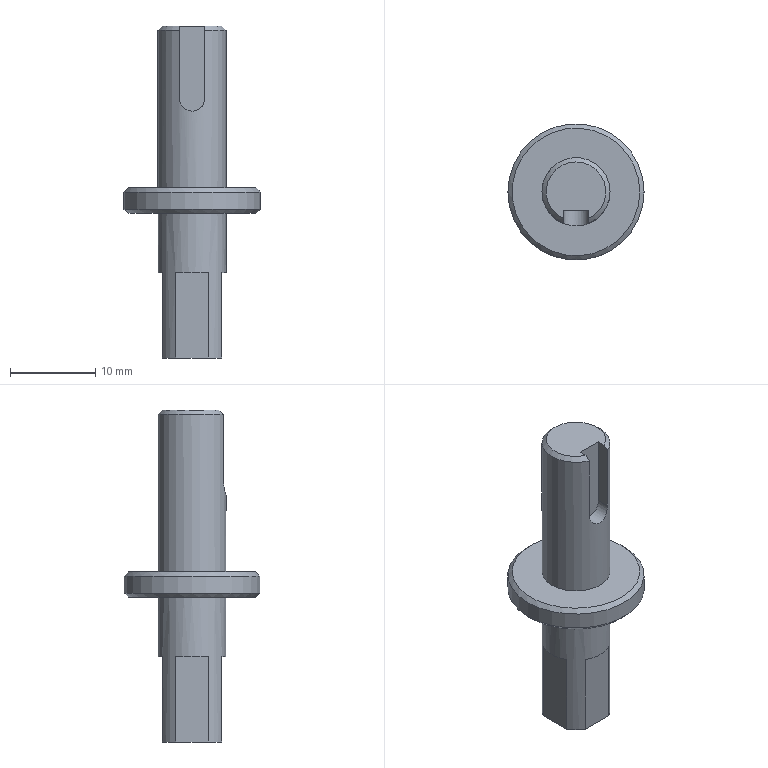Part | NX | features DATUM_CSYS 2, EXTRUDE 2, BREP 1, SKETCH 1 | 1 solid | 25 faces | box 16 x 16 x 39 mm | volume 2221 mm3 | plane 15 | cylinder 6 | cone 4 | commonest cylinder face diameters 2.5 x2 8 x2 3 x1 16 x1
STEP:
#1=CARTESIAN_POINT('',(-3.5,1.936,-20.));
#2=VERTEX_POINT('',#1);
#3=CARTESIAN_POINT('',(-1.936,3.5,-20.));
#4=VERTEX_POINT('',#3);
#5=CARTESIAN_POINT('',(0.,0.,-20.));
#6=DIRECTION('',(0.,0.,-1.));
#7=DIRECTION('',(1.,0.,0.));
#8=AXIS2_PLACEMENT_3D('',#5,#6,#7);
#9=CIRCLE('',#8,4.);
#10=EDGE_CURVE('',#2,#4,#9,.T.);
#11=ORIENTED_EDGE('',*,*,#10,.F.);
#12=CARTESIAN_POINT('',(-3.5,1.936,-10.));
#13=VERTEX_POINT('',#12);
#14=CARTESIAN_POINT('',(-3.5,1.936,-10.));
#15=DIRECTION('',(0.,0.,-1.));
#16=VECTOR('',#15,1000.);
#17=LINE('',#14,#16);
#18=EDGE_CURVE('',#13,#2,#17,.T.);
#19=ORIENTED_EDGE('',*,*,#18,.F.);
#20=CARTESIAN_POINT('',(-3.5,-1.936,-10.));
#21=VERTEX_POINT('',#20);
#22=CARTESIAN_POINT('',(0.,0.,-10.));
#23=DIRECTION('',(0.,0.,-1.));
#24=DIRECTION('',(-0.875,-0.4841,0.));
#25=AXIS2_PLACEMENT_3D('',#22,#23,#24);
#26=CIRCLE('',#25,4.);
#27=EDGE_CURVE('',#21,#13,#26,.T.);
#28=ORIENTED_EDGE('',*,*,#27,.F.);
#29=CARTESIAN_POINT('',(-3.5,-1.936,-20.));
#30=VERTEX_POINT('',#29);
#31=CARTESIAN_POINT('',(-3.5,-1.936,-14.5));
#32=DIRECTION('',(0.,0.,1.));
#33=VECTOR('',#32,1000.);
#34=LINE('',#31,#33);
#35=EDGE_CURVE('',#30,#21,#34,.T.);
#36=ORIENTED_EDGE('',*,*,#35,.F.);
#37=CARTESIAN_POINT('',(-1.936,-3.5,-20.));
#38=VERTEX_POINT('',#37);
#39=CARTESIAN_POINT('',(0.,0.,-20.));
#40=DIRECTION('',(0.,0.,-1.));
#41=DIRECTION('',(1.,0.,0.));
#42=AXIS2_PLACEMENT_3D('',#39,#40,#41);
#43=CIRCLE('',#42,4.);
#44=EDGE_CURVE('',#38,#30,#43,.T.);
#45=ORIENTED_EDGE('',*,*,#44,.F.);
#46=CARTESIAN_POINT('',(-1.936,-3.5,-10.));
#47=VERTEX_POINT('',#46);
#48=CARTESIAN_POINT('',(-1.936,-3.5,-10.));
#49=DIRECTION('',(0.,0.,-1.));
#50=VECTOR('',#49,1000.);
#51=LINE('',#48,#50);
#52=EDGE_CURVE('',#47,#38,#51,.T.);
#53=ORIENTED_EDGE('',*,*,#52,.F.);
#54=CARTESIAN_POINT('',(1.936,-3.5,-10.));
#55=VERTEX_POINT('',#54);
#56=CARTESIAN_POINT('',(0.,0.,-10.));
#57=DIRECTION('',(0.,0.,-1.));
#58=DIRECTION('',(0.4841,-0.875,0.));
#59=AXIS2_PLACEMENT_3D('',#56,#57,#58);
#60=CIRCLE('',#59,4.);
#61=EDGE_CURVE('',#55,#47,#60,.T.);
#62=ORIENTED_EDGE('',*,*,#61,.F.);
#63=CARTESIAN_POINT('',(1.936,-3.5,-20.));
#64=VERTEX_POINT('',#63);
#65=CARTESIAN_POINT('',(1.936,-3.5,-14.5));
#66=DIRECTION('',(0.,0.,1.));
#67=VECTOR('',#66,1000.);
#68=LINE('',#65,#67);
#69=EDGE_CURVE('',#64,#55,#68,.T.);
#70=ORIENTED_EDGE('',*,*,#69,.F.);
#71=CARTESIAN_POINT('',(3.5,-1.936,-20.));
#72=VERTEX_POINT('',#71);
#73=CARTESIAN_POINT('',(0.,0.,-20.));
#74=DIRECTION('',(0.,0.,-1.));
#75=DIRECTION('',(1.,0.,0.));
#76=AXIS2_PLACEMENT_3D('',#73,#74,#75);
#77=CIRCLE('',#76,4.);
#78=EDGE_CURVE('',#72,#64,#77,.T.);
#79=ORIENTED_EDGE('',*,*,#78,.F.);
#80=CARTESIAN_POINT('',(3.5,-1.936,-10.));
#81=VERTEX_POINT('',#80);
#82=CARTESIAN_POINT('',(3.5,-1.936,-10.));
#83=DIRECTION('',(0.,0.,-1.));
#84=VECTOR('',#83,1000.);
#85=LINE('',#82,#84);
#86=EDGE_CURVE('',#81,#72,#85,.T.);
#87=ORIENTED_EDGE('',*,*,#86,.F.);
#88=CARTESIAN_POINT('',(4.,0.,-10.));
#89=VERTEX_POINT('',#88);
#90=CARTESIAN_POINT('',(0.,0.,-10.));
#91=DIRECTION('',(0.,0.,-1.));
#92=DIRECTION('',(1.,0.,0.));
#93=AXIS2_PLACEMENT_3D('',#90,#91,#92);
#94=CIRCLE('',#93,4.);
#95=EDGE_CURVE('',#89,#81,#94,.T.);
#96=ORIENTED_EDGE('',*,*,#95,.F.);
#97=CARTESIAN_POINT('',(4.,0.,-3.));
#98=VERTEX_POINT('',#97);
#99=CARTESIAN_POINT('',(4.,0.,-3.));
#100=DIRECTION('',(0.,0.,-1.));
#101=VECTOR('',#100,1000.);
#102=LINE('',#99,#101);
#103=EDGE_CURVE('',#98,#89,#102,.T.);
#104=ORIENTED_EDGE('',*,*,#103,.F.);
#105=CARTESIAN_POINT('',(0.,0.,-3.));
#106=DIRECTION('',(0.,0.,-1.));
#107=DIRECTION('',(1.,0.,0.));
#108=AXIS2_PLACEMENT_3D('',#105,#106,#107);
#109=CIRCLE('',#108,4.);
#110=EDGE_CURVE('',#98,#98,#109,.T.);
#111=ORIENTED_EDGE('',*,*,#110,.T.);
#112=ORIENTED_EDGE('',*,*,#103,.T.);
#113=CARTESIAN_POINT('',(3.5,1.936,-10.));
#114=VERTEX_POINT('',#113);
#115=CARTESIAN_POINT('',(0.,0.,-10.));
#116=DIRECTION('',(0.,0.,-1.));
#117=DIRECTION('',(0.875,0.4841,0.));
#118=AXIS2_PLACEMENT_3D('',#115,#116,#117);
#119=CIRCLE('',#118,4.);
#120=EDGE_CURVE('',#114,#89,#119,.T.);
#121=ORIENTED_EDGE('',*,*,#120,.F.);
#122=CARTESIAN_POINT('',(3.5,1.936,-20.));
#123=VERTEX_POINT('',#122);
#124=CARTESIAN_POINT('',(3.5,1.936,-14.5));
#125=DIRECTION('',(0.,0.,1.));
#126=VECTOR('',#125,1000.);
#127=LINE('',#124,#126);
#128=EDGE_CURVE('',#123,#114,#127,.T.);
#129=ORIENTED_EDGE('',*,*,#128,.F.);
#130=CARTESIAN_POINT('',(1.936,3.5,-20.));
#131=VERTEX_POINT('',#130);
#132=CARTESIAN_POINT('',(0.,0.,-20.));
#133=DIRECTION('',(0.,0.,-1.));
#134=DIRECTION('',(1.,0.,0.));
#135=AXIS2_PLACEMENT_3D('',#132,#133,#134);
#136=CIRCLE('',#135,4.);
#137=EDGE_CURVE('',#131,#123,#136,.T.);
#138=ORIENTED_EDGE('',*,*,#137,.F.);
#139=CARTESIAN_POINT('',(1.936,3.5,-10.));
#140=VERTEX_POINT('',#139);
#141=CARTESIAN_POINT('',(1.936,3.5,-10.));
#142=DIRECTION('',(0.,0.,-1.));
#143=VECTOR('',#142,1000.);
#144=LINE('',#141,#143);
#145=EDGE_CURVE('',#140,#131,#144,.T.);
#146=ORIENTED_EDGE('',*,*,#145,.F.);
#147=CARTESIAN_POINT('',(-1.936,3.5,-10.));
#148=VERTEX_POINT('',#147);
#149=CARTESIAN_POINT('',(0.,0.,-10.));
#150=DIRECTION('',(0.,0.,-1.));
#151=DIRECTION('',(-0.4841,0.875,0.));
#152=AXIS2_PLACEMENT_3D('',#149,#150,#151);
#153=CIRCLE('',#152,4.);
#154=EDGE_CURVE('',#148,#140,#153,.T.);
#155=ORIENTED_EDGE('',*,*,#154,.F.);
#156=CARTESIAN_POINT('',(-1.936,3.5,-14.5));
#157=DIRECTION('',(0.,0.,1.));
#158=VECTOR('',#157,1000.);
#159=LINE('',#156,#158);
#160=EDGE_CURVE('',#4,#148,#159,.T.);
#161=ORIENTED_EDGE('',*,*,#160,.F.);
#162=EDGE_LOOP('',(#11,#19,#28,#36,#45,#53,#62,#70,#79,#87,#96,#104,#111,#112,#121,#129,#138,#146,#155,#161));
#163=FACE_BOUND('',#162,.T.);
#164=CARTESIAN_POINT('',(0.,0.,-3.));
#165=DIRECTION('',(0.,0.,-1.));
#166=DIRECTION('',(-1.,0.,0.));
#167=AXIS2_PLACEMENT_3D('',#164,#165,#166);
#168=CYLINDRICAL_SURFACE('',#167,4.);
#169=ADVANCED_FACE('',(#163),#168,.T.);
#170=ORIENTED_EDGE('',*,*,#86,.T.);
#171=CARTESIAN_POINT('',(3.5,0.,-20.));
#172=DIRECTION('',(0.,-1.,0.));
#173=VECTOR('',#172,1000.);
#174=LINE('',#171,#173);
#175=EDGE_CURVE('',#123,#72,#174,.T.);
#176=ORIENTED_EDGE('',*,*,#175,.F.);
#177=ORIENTED_EDGE('',*,*,#128,.T.);
#178=CARTESIAN_POINT('',(3.5,-1.936,-10.));
#179=DIRECTION('',(0.,1.,0.));
#180=VECTOR('',#179,1000.);
#181=LINE('',#178,#180);
#182=EDGE_CURVE('',#81,#114,#181,.T.);
#183=ORIENTED_EDGE('',*,*,#182,.F.);
#184=EDGE_LOOP('',(#170,#176,#177,#183));
#185=FACE_BOUND('',#184,.T.);
#186=CARTESIAN_POINT('',(3.5,0.,-12.5));
#187=DIRECTION('',(1.,0.,0.));
#188=DIRECTION('',(0.,-1.,0.));
#189=AXIS2_PLACEMENT_3D('',#186,#187,#188);
#190=PLANE('',#189);
#191=ADVANCED_FACE('',(#185),#190,.T.);
#192=ORIENTED_EDGE('',*,*,#145,.T.);
#193=CARTESIAN_POINT('',(0.,3.5,-20.));
#194=DIRECTION('',(1.,0.,0.));
#195=VECTOR('',#194,1000.);
#196=LINE('',#193,#195);
#197=EDGE_CURVE('',#4,#131,#196,.T.);
#198=ORIENTED_EDGE('',*,*,#197,.F.);
#199=ORIENTED_EDGE('',*,*,#160,.T.);
#200=CARTESIAN_POINT('',(1.936,3.5,-10.));
#201=DIRECTION('',(-1.,0.,0.));
#202=VECTOR('',#201,1000.);
#203=LINE('',#200,#202);
#204=EDGE_CURVE('',#140,#148,#203,.T.);
#205=ORIENTED_EDGE('',*,*,#204,.F.);
#206=EDGE_LOOP('',(#192,#198,#199,#205));
#207=FACE_BOUND('',#206,.T.);
#208=CARTESIAN_POINT('',(0.,3.5,-12.5));
#209=DIRECTION('',(0.,1.,0.));
#210=DIRECTION('',(1.,0.,0.));
#211=AXIS2_PLACEMENT_3D('',#208,#209,#210);
#212=PLANE('',#211);
#213=ADVANCED_FACE('',(#207),#212,.T.);
#214=ORIENTED_EDGE('',*,*,#18,.T.);
#215=CARTESIAN_POINT('',(-3.5,0.,-20.));
#216=DIRECTION('',(0.,1.,0.));
#217=VECTOR('',#216,1000.);
#218=LINE('',#215,#217);
#219=EDGE_CURVE('',#30,#2,#218,.T.);
#220=ORIENTED_EDGE('',*,*,#219,.F.);
#221=ORIENTED_EDGE('',*,*,#35,.T.);
#222=CARTESIAN_POINT('',(-3.5,1.936,-10.));
#223=DIRECTION('',(0.,-1.,0.));
#224=VECTOR('',#223,1000.);
#225=LINE('',#222,#224);
#226=EDGE_CURVE('',#13,#21,#225,.T.);
#227=ORIENTED_EDGE('',*,*,#226,.F.);
#228=EDGE_LOOP('',(#214,#220,#221,#227));
#229=FACE_BOUND('',#228,.T.);
#230=CARTESIAN_POINT('',(-3.5,0.,-12.5));
#231=DIRECTION('',(-1.,0.,0.));
#232=DIRECTION('',(0.,1.,0.));
#233=AXIS2_PLACEMENT_3D('',#230,#231,#232);
#234=PLANE('',#233);
#235=ADVANCED_FACE('',(#229),#234,.T.);
#236=ORIENTED_EDGE('',*,*,#52,.T.);
#237=CARTESIAN_POINT('',(0.,-3.5,-20.));
#238=DIRECTION('',(-1.,0.,0.));
#239=VECTOR('',#238,1000.);
#240=LINE('',#237,#239);
#241=EDGE_CURVE('',#64,#38,#240,.T.);
#242=ORIENTED_EDGE('',*,*,#241,.F.);
#243=ORIENTED_EDGE('',*,*,#69,.T.);
#244=CARTESIAN_POINT('',(-1.936,-3.5,-10.));
#245=DIRECTION('',(1.,0.,0.));
#246=VECTOR('',#245,1000.);
#247=LINE('',#244,#246);
#248=EDGE_CURVE('',#47,#55,#247,.T.);
#249=ORIENTED_EDGE('',*,*,#248,.F.);
#250=EDGE_LOOP('',(#236,#242,#243,#249));
#251=FACE_BOUND('',#250,.T.);
#252=CARTESIAN_POINT('',(0.,-3.5,-12.5));
#253=DIRECTION('',(0.,-1.,0.));
#254=DIRECTION('',(-1.,0.,0.));
#255=AXIS2_PLACEMENT_3D('',#252,#253,#254);
#256=PLANE('',#255);
#257=ADVANCED_FACE('',(#251),#256,.T.);
#258=CARTESIAN_POINT('',(7.5,0.,-3.));
#259=VERTEX_POINT('',#258);
#260=CARTESIAN_POINT('',(0.,0.,-3.));
#261=DIRECTION('',(0.,0.,1.));
#262=DIRECTION('',(1.,0.,0.));
#263=AXIS2_PLACEMENT_3D('',#260,#261,#262);
#264=CIRCLE('',#263,7.5);
#265=EDGE_CURVE('',#259,#259,#264,.T.);
#266=ORIENTED_EDGE('',*,*,#265,.F.);
#267=EDGE_LOOP('',(#266));
#268=FACE_BOUND('',#267,.T.);
#269=ORIENTED_EDGE('',*,*,#110,.F.);
#270=EDGE_LOOP('',(#269));
#271=FACE_BOUND('',#270,.T.);
#272=CARTESIAN_POINT('',(0.,0.,-3.));
#273=DIRECTION('',(0.,0.,-1.));
#274=DIRECTION('',(-1.,0.,0.));
#275=AXIS2_PLACEMENT_3D('',#272,#273,#274);
#276=PLANE('',#275);
#277=ADVANCED_FACE('',(#268,#271),#276,.T.);
#278=CARTESIAN_POINT('',(8.,0.,-0.5));
#279=VERTEX_POINT('',#278);
#280=CARTESIAN_POINT('',(8.,0.,-2.5));
#281=VERTEX_POINT('',#280);
#282=CARTESIAN_POINT('',(8.,0.,-0.5));
#283=DIRECTION('',(0.,0.,-1.));
#284=VECTOR('',#283,1000.);
#285=LINE('',#282,#284);
#286=EDGE_CURVE('',#279,#281,#285,.T.);
#287=ORIENTED_EDGE('',*,*,#286,.F.);
#288=CARTESIAN_POINT('',(0.,0.,-0.5));
#289=DIRECTION('',(0.,0.,1.));
#290=DIRECTION('',(1.,0.,0.));
#291=AXIS2_PLACEMENT_3D('',#288,#289,#290);
#292=CIRCLE('',#291,8.);
#293=EDGE_CURVE('',#279,#279,#292,.T.);
#294=ORIENTED_EDGE('',*,*,#293,.F.);
#295=ORIENTED_EDGE('',*,*,#286,.T.);
#296=CARTESIAN_POINT('',(0.,0.,-2.5));
#297=DIRECTION('',(0.,0.,1.));
#298=DIRECTION('',(1.,0.,0.));
#299=AXIS2_PLACEMENT_3D('',#296,#297,#298);
#300=CIRCLE('',#299,8.);
#301=EDGE_CURVE('',#281,#281,#300,.T.);
#302=ORIENTED_EDGE('',*,*,#301,.T.);
#303=EDGE_LOOP('',(#287,#294,#295,#302));
#304=FACE_BOUND('',#303,.T.);
#305=CARTESIAN_POINT('',(0.,0.,0.));
#306=DIRECTION('',(0.,0.,-1.));
#307=DIRECTION('',(-1.,0.,0.));
#308=AXIS2_PLACEMENT_3D('',#305,#306,#307);
#309=CYLINDRICAL_SURFACE('',#308,8.);
#310=ADVANCED_FACE('',(#304),#309,.T.);
#311=CARTESIAN_POINT('',(7.5,0.,0.));
#312=VERTEX_POINT('',#311);
#313=CARTESIAN_POINT('',(0.,0.,0.));
#314=DIRECTION('',(0.,0.,1.));
#315=DIRECTION('',(1.,0.,0.));
#316=AXIS2_PLACEMENT_3D('',#313,#314,#315);
#317=CIRCLE('',#316,7.5);
#318=EDGE_CURVE('',#312,#312,#317,.T.);
#319=ORIENTED_EDGE('',*,*,#318,.T.);
#320=EDGE_LOOP('',(#319));
#321=FACE_BOUND('',#320,.T.);
#322=CARTESIAN_POINT('',(4.,0.,0.));
#323=VERTEX_POINT('',#322);
#324=CARTESIAN_POINT('',(0.,0.,0.));
#325=DIRECTION('',(0.,0.,1.));
#326=DIRECTION('',(1.,0.,0.));
#327=AXIS2_PLACEMENT_3D('',#324,#325,#326);
#328=CIRCLE('',#327,4.);
#329=EDGE_CURVE('',#323,#323,#328,.T.);
#330=ORIENTED_EDGE('',*,*,#329,.F.);
#331=EDGE_LOOP('',(#330));
#332=FACE_BOUND('',#331,.T.);
#333=CARTESIAN_POINT('',(0.,0.,0.));
#334=DIRECTION('',(0.,0.,-1.));
#335=DIRECTION('',(-1.,0.,0.));
#336=AXIS2_PLACEMENT_3D('',#333,#334,#335);
#337=PLANE('',#336);
#338=ADVANCED_FACE('',(#321,#332),#337,.F.);
#339=ORIENTED_EDGE('',*,*,#329,.T.);
#340=CARTESIAN_POINT('',(4.,0.,18.5));
#341=VERTEX_POINT('',#340);
#342=CARTESIAN_POINT('',(4.,0.,0.));
#343=DIRECTION('',(0.,0.,1.));
#344=VECTOR('',#343,1000.);
#345=LINE('',#342,#344);
#346=EDGE_CURVE('',#323,#341,#345,.T.);
#347=ORIENTED_EDGE('',*,*,#346,.T.);
#348=CARTESIAN_POINT('',(1.5,-3.708,18.5));
#349=VERTEX_POINT('',#348);
#350=CARTESIAN_POINT('',(0.,0.,18.5));
#351=DIRECTION('',(0.,0.,-1.));
#352=DIRECTION('',(1.,0.,0.));
#353=AXIS2_PLACEMENT_3D('',#350,#351,#352);
#354=CIRCLE('',#353,4.);
#355=EDGE_CURVE('',#341,#349,#354,.T.);
#356=ORIENTED_EDGE('',*,*,#355,.T.);
#357=CARTESIAN_POINT('',(1.5,-3.708,10.5));
#358=VERTEX_POINT('',#357);
#359=CARTESIAN_POINT('',(1.5,-3.708,10.5));
#360=DIRECTION('',(0.,0.,1.));
#361=VECTOR('',#360,1000.);
#362=LINE('',#359,#361);
#363=EDGE_CURVE('',#358,#349,#362,.T.);
#364=ORIENTED_EDGE('',*,*,#363,.F.);
#365=CARTESIAN_POINT('',(-1.5,-3.708,10.5));
#366=VERTEX_POINT('',#365);
#367=CARTESIAN_POINT('',(-1.5,-3.708,10.5));
#368=CARTESIAN_POINT('',(-1.5,-3.708,10.1));
#369=CARTESIAN_POINT('',(-1.175,-3.859,9.329));
#370=CARTESIAN_POINT('',(-0.002874,-4.07,8.836));
#371=CARTESIAN_POINT('',(1.176,-3.86,9.329));
#372=CARTESIAN_POINT('',(1.5,-3.708,10.1));
#373=CARTESIAN_POINT('',(1.5,-3.708,10.5));
#374=B_SPLINE_CURVE_WITH_KNOTS('',3,(#367,#368,#369,#370,#371,#372,#373),.UNSPECIFIED.,.F.,.F.,(4,1,1,1,4),(0.,0.001183,0.002366,0.003548,0.004731),.UNSPECIFIED.);
#375=EDGE_CURVE('',#366,#358,#374,.T.);
#376=ORIENTED_EDGE('',*,*,#375,.F.);
#377=CARTESIAN_POINT('',(-1.5,-3.708,18.5));
#378=VERTEX_POINT('',#377);
#379=CARTESIAN_POINT('',(-1.5,-3.708,18.5));
#380=DIRECTION('',(0.,0.,-1.));
#381=VECTOR('',#380,1000.);
#382=LINE('',#379,#381);
#383=EDGE_CURVE('',#378,#366,#382,.T.);
#384=ORIENTED_EDGE('',*,*,#383,.F.);
#385=CARTESIAN_POINT('',(0.,0.,18.5));
#386=DIRECTION('',(0.,0.,-1.));
#387=DIRECTION('',(-0.375,-0.927,0.));
#388=AXIS2_PLACEMENT_3D('',#385,#386,#387);
#389=CIRCLE('',#388,4.);
#390=EDGE_CURVE('',#378,#341,#389,.T.);
#391=ORIENTED_EDGE('',*,*,#390,.T.);
#392=ORIENTED_EDGE('',*,*,#346,.F.);
#393=EDGE_LOOP('',(#339,#347,#356,#364,#376,#384,#391,#392));
#394=FACE_BOUND('',#393,.T.);
#395=CARTESIAN_POINT('',(0.,0.,0.));
#396=DIRECTION('',(0.,0.,1.));
#397=DIRECTION('',(-1.,0.,0.));
#398=AXIS2_PLACEMENT_3D('',#395,#396,#397);
#399=CYLINDRICAL_SURFACE('',#398,4.);
#400=ADVANCED_FACE('',(#394),#399,.T.);
#401=CARTESIAN_POINT('',(1.5,-3.162,19.));
#402=VERTEX_POINT('',#401);
#403=CARTESIAN_POINT('',(-1.5,-3.162,19.));
#404=VERTEX_POINT('',#403);
#405=CARTESIAN_POINT('',(0.,0.,19.));
#406=DIRECTION('',(0.,0.,1.));
#407=DIRECTION('',(0.4286,-0.9035,0.));
#408=AXIS2_PLACEMENT_3D('',#405,#406,#407);
#409=CIRCLE('',#408,3.5);
#410=EDGE_CURVE('',#402,#404,#409,.T.);
#411=ORIENTED_EDGE('',*,*,#410,.T.);
#412=CARTESIAN_POINT('',(-1.5,-2.2,19.));
#413=VERTEX_POINT('',#412);
#414=CARTESIAN_POINT('',(-1.5,-2.2,19.));
#415=DIRECTION('',(0.,-1.,0.));
#416=VECTOR('',#415,1000.);
#417=LINE('',#414,#416);
#418=EDGE_CURVE('',#413,#404,#417,.T.);
#419=ORIENTED_EDGE('',*,*,#418,.F.);
#420=CARTESIAN_POINT('',(1.5,-2.2,19.));
#421=VERTEX_POINT('',#420);
#422=CARTESIAN_POINT('',(1.5,-2.2,19.));
#423=DIRECTION('',(-1.,0.,0.));
#424=VECTOR('',#423,1000.);
#425=LINE('',#422,#424);
#426=EDGE_CURVE('',#421,#413,#425,.T.);
#427=ORIENTED_EDGE('',*,*,#426,.F.);
#428=CARTESIAN_POINT('',(1.5,-3.162,19.));
#429=DIRECTION('',(0.,1.,0.));
#430=VECTOR('',#429,1000.);
#431=LINE('',#428,#430);
#432=EDGE_CURVE('',#402,#421,#431,.T.);
#433=ORIENTED_EDGE('',*,*,#432,.F.);
#434=EDGE_LOOP('',(#411,#419,#427,#433));
#435=FACE_BOUND('',#434,.T.);
#436=CARTESIAN_POINT('',(0.,0.,19.));
#437=DIRECTION('',(0.,0.,1.));
#438=DIRECTION('',(-1.,0.,0.));
#439=AXIS2_PLACEMENT_3D('',#436,#437,#438);
#440=PLANE('',#439);
#441=ADVANCED_FACE('',(#435),#440,.T.);
#442=ORIENTED_EDGE('',*,*,#390,.F.);
#443=CARTESIAN_POINT('',(-1.5,-3.162,19.));
#444=CARTESIAN_POINT('',(-1.5,-3.417,18.77));
#445=CARTESIAN_POINT('',(-1.5,-3.708,18.5));
#446=(BOUNDED_CURVE()B_SPLINE_CURVE(2,(#443,#444,#445),.UNSPECIFIED.,.F.,.F.)B_SPLINE_CURVE_WITH_KNOTS((3,3),(0.,1.),.PIECEWISE_BEZIER_KNOTS.)CURVE()GEOMETRIC_REPRESENTATION_ITEM()RATIONAL_B_SPLINE_CURVE((1.1,1.052,1.))REPRESENTATION_ITEM(''));
#447=EDGE_CURVE('',#404,#378,#446,.T.);
#448=ORIENTED_EDGE('',*,*,#447,.F.);
#449=ORIENTED_EDGE('',*,*,#410,.F.);
#450=CARTESIAN_POINT('',(1.5,-3.708,18.5));
#451=CARTESIAN_POINT('',(1.5,-3.417,18.77));
#452=CARTESIAN_POINT('',(1.5,-3.162,19.));
#453=(BOUNDED_CURVE()B_SPLINE_CURVE(2,(#450,#451,#452),.UNSPECIFIED.,.F.,.F.)B_SPLINE_CURVE_WITH_KNOTS((3,3),(0.,1.),.PIECEWISE_BEZIER_KNOTS.)CURVE()GEOMETRIC_REPRESENTATION_ITEM()RATIONAL_B_SPLINE_CURVE((1.,1.052,1.1))REPRESENTATION_ITEM(''));
#454=EDGE_CURVE('',#349,#402,#453,.T.);
#455=ORIENTED_EDGE('',*,*,#454,.F.);
#456=ORIENTED_EDGE('',*,*,#355,.F.);
#457=EDGE_LOOP('',(#442,#448,#449,#455,#456));
#458=FACE_BOUND('',#457,.T.);
#459=CARTESIAN_POINT('',(0.,0.,19.));
#460=DIRECTION('',(0.,0.,-1.));
#461=DIRECTION('',(0.375,0.927,0.));
#462=AXIS2_PLACEMENT_3D('',#459,#460,#461);
#463=CONICAL_SURFACE('',#462,3.5,0.7854);
#464=ADVANCED_FACE('',(#458),#463,.T.);
#465=CARTESIAN_POINT('',(7.5,0.,-3.));
#466=DIRECTION('',(0.7071,0.,0.7071));
#467=VECTOR('',#466,1000.);
#468=LINE('',#465,#467);
#469=EDGE_CURVE('',#259,#281,#468,.T.);
#470=ORIENTED_EDGE('',*,*,#469,.T.);
#471=ORIENTED_EDGE('',*,*,#301,.F.);
#472=ORIENTED_EDGE('',*,*,#469,.F.);
#473=ORIENTED_EDGE('',*,*,#265,.T.);
#474=EDGE_LOOP('',(#470,#471,#472,#473));
#475=FACE_BOUND('',#474,.T.);
#476=CARTESIAN_POINT('',(0.,0.,-3.));
#477=DIRECTION('',(0.,0.,1.));
#478=DIRECTION('',(-1.,0.,0.));
#479=AXIS2_PLACEMENT_3D('',#476,#477,#478);
#480=CONICAL_SURFACE('',#479,7.5,0.7854);
#481=ADVANCED_FACE('',(#475),#480,.T.);
#482=ORIENTED_EDGE('',*,*,#318,.F.);
#483=CARTESIAN_POINT('',(7.5,0.,0.));
#484=DIRECTION('',(0.7071,0.,-0.7071));
#485=VECTOR('',#484,1000.);
#486=LINE('',#483,#485);
#487=EDGE_CURVE('',#312,#279,#486,.T.);
#488=ORIENTED_EDGE('',*,*,#487,.T.);
#489=ORIENTED_EDGE('',*,*,#293,.T.);
#490=ORIENTED_EDGE('',*,*,#487,.F.);
#491=EDGE_LOOP('',(#482,#488,#489,#490));
#492=FACE_BOUND('',#491,.T.);
#493=CARTESIAN_POINT('',(0.,0.,0.));
#494=DIRECTION('',(0.,0.,-1.));
#495=DIRECTION('',(-1.,0.,0.));
#496=AXIS2_PLACEMENT_3D('',#493,#494,#495);
#497=CONICAL_SURFACE('',#496,7.5,0.7854);
#498=ADVANCED_FACE('',(#492),#497,.T.);
#499=CARTESIAN_POINT('',(1.5,-2.2,10.5));
#500=VERTEX_POINT('',#499);
#501=CARTESIAN_POINT('',(1.5,-2.2,10.5));
#502=DIRECTION('',(0.,-1.,0.));
#503=VECTOR('',#502,1000.);
#504=LINE('',#501,#503);
#505=EDGE_CURVE('',#500,#358,#504,.T.);
#506=ORIENTED_EDGE('',*,*,#505,.T.);
#507=ORIENTED_EDGE('',*,*,#363,.T.);
#508=ORIENTED_EDGE('',*,*,#454,.T.);
#509=ORIENTED_EDGE('',*,*,#432,.T.);
#510=CARTESIAN_POINT('',(1.5,-2.2,10.5));
#511=DIRECTION('',(0.,0.,1.));
#512=VECTOR('',#511,1000.);
#513=LINE('',#510,#512);
#514=EDGE_CURVE('',#500,#421,#513,.T.);
#515=ORIENTED_EDGE('',*,*,#514,.F.);
#516=EDGE_LOOP('',(#506,#507,#508,#509,#515));
#517=FACE_BOUND('',#516,.T.);
#518=CARTESIAN_POINT('',(1.5,-5.165,15.5));
#519=DIRECTION('',(1.,0.,0.));
#520=DIRECTION('',(0.,0.,-1.));
#521=AXIS2_PLACEMENT_3D('',#518,#519,#520);
#522=PLANE('',#521);
#523=ADVANCED_FACE('',(#517),#522,.F.);
#524=CARTESIAN_POINT('',(-1.5,-2.2,10.5));
#525=VERTEX_POINT('',#524);
#526=CARTESIAN_POINT('',(-1.5,-2.2,10.5));
#527=DIRECTION('',(0.,-1.,0.));
#528=VECTOR('',#527,1000.);
#529=LINE('',#526,#528);
#530=EDGE_CURVE('',#525,#366,#529,.T.);
#531=ORIENTED_EDGE('',*,*,#530,.T.);
#532=ORIENTED_EDGE('',*,*,#375,.T.);
#533=ORIENTED_EDGE('',*,*,#505,.F.);
#534=CARTESIAN_POINT('',(0.,-2.2,10.5));
#535=DIRECTION('',(0.,-1.,0.));
#536=DIRECTION('',(-1.,0.,0.));
#537=AXIS2_PLACEMENT_3D('',#534,#535,#536);
#538=CIRCLE('',#537,1.5);
#539=EDGE_CURVE('',#525,#500,#538,.T.);
#540=ORIENTED_EDGE('',*,*,#539,.F.);
#541=EDGE_LOOP('',(#531,#532,#533,#540));
#542=FACE_BOUND('',#541,.T.);
#543=CARTESIAN_POINT('',(0.,-2.2,10.5));
#544=DIRECTION('',(0.,-1.,0.));
#545=DIRECTION('',(1.,0.,0.));
#546=AXIS2_PLACEMENT_3D('',#543,#544,#545);
#547=CYLINDRICAL_SURFACE('',#546,1.5);
#548=ADVANCED_FACE('',(#542),#547,.F.);
#549=CARTESIAN_POINT('',(-1.5,-2.2,19.));
#550=DIRECTION('',(0.,0.,-1.));
#551=VECTOR('',#550,1000.);
#552=LINE('',#549,#551);
#553=EDGE_CURVE('',#413,#525,#552,.T.);
#554=ORIENTED_EDGE('',*,*,#553,.F.);
#555=ORIENTED_EDGE('',*,*,#418,.T.);
#556=ORIENTED_EDGE('',*,*,#447,.T.);
#557=ORIENTED_EDGE('',*,*,#383,.T.);
#558=ORIENTED_EDGE('',*,*,#530,.F.);
#559=EDGE_LOOP('',(#554,#555,#556,#557,#558));
#560=FACE_BOUND('',#559,.T.);
#561=CARTESIAN_POINT('',(-1.5,-5.165,15.5));
#562=DIRECTION('',(-1.,0.,0.));
#563=DIRECTION('',(0.,0.,1.));
#564=AXIS2_PLACEMENT_3D('',#561,#562,#563);
#565=PLANE('',#564);
#566=ADVANCED_FACE('',(#560),#565,.F.);
#567=ORIENTED_EDGE('',*,*,#539,.T.);
#568=ORIENTED_EDGE('',*,*,#514,.T.);
#569=ORIENTED_EDGE('',*,*,#426,.T.);
#570=ORIENTED_EDGE('',*,*,#553,.T.);
#571=EDGE_LOOP('',(#567,#568,#569,#570));
#572=FACE_BOUND('',#571,.T.);
#573=CARTESIAN_POINT('',(5.,-2.2,15.5));
#574=DIRECTION('',(0.,-1.,0.));
#575=DIRECTION('',(-1.,0.,0.));
#576=AXIS2_PLACEMENT_3D('',#573,#574,#575);
#577=PLANE('',#576);
#578=ADVANCED_FACE('',(#572),#577,.T.);
#579=ORIENTED_EDGE('',*,*,#182,.T.);
#580=ORIENTED_EDGE('',*,*,#120,.T.);
#581=ORIENTED_EDGE('',*,*,#95,.T.);
#582=EDGE_LOOP('',(#579,#580,#581));
#583=FACE_BOUND('',#582,.T.);
#584=CARTESIAN_POINT('',(3.75,0.,-10.));
#585=DIRECTION('',(0.,0.,-1.));
#586=DIRECTION('',(-1.,0.,0.));
#587=AXIS2_PLACEMENT_3D('',#584,#585,#586);
#588=PLANE('',#587);
#589=ADVANCED_FACE('',(#583),#588,.T.);
#590=ORIENTED_EDGE('',*,*,#204,.T.);
#591=ORIENTED_EDGE('',*,*,#154,.T.);
#592=EDGE_LOOP('',(#590,#591));
#593=FACE_BOUND('',#592,.T.);
#594=CARTESIAN_POINT('',(0.,3.75,-10.));
#595=DIRECTION('',(0.,0.,-1.));
#596=DIRECTION('',(-1.,0.,0.));
#597=AXIS2_PLACEMENT_3D('',#594,#595,#596);
#598=PLANE('',#597);
#599=ADVANCED_FACE('',(#593),#598,.T.);
#600=ORIENTED_EDGE('',*,*,#226,.T.);
#601=ORIENTED_EDGE('',*,*,#27,.T.);
#602=EDGE_LOOP('',(#600,#601));
#603=FACE_BOUND('',#602,.T.);
#604=CARTESIAN_POINT('',(-3.75,0.,-10.));
#605=DIRECTION('',(0.,0.,-1.));
#606=DIRECTION('',(-1.,0.,0.));
#607=AXIS2_PLACEMENT_3D('',#604,#605,#606);
#608=PLANE('',#607);
#609=ADVANCED_FACE('',(#603),#608,.T.);
#610=ORIENTED_EDGE('',*,*,#248,.T.);
#611=ORIENTED_EDGE('',*,*,#61,.T.);
#612=EDGE_LOOP('',(#610,#611));
#613=FACE_BOUND('',#612,.T.);
#614=CARTESIAN_POINT('',(0.,-3.75,-10.));
#615=DIRECTION('',(0.,0.,-1.));
#616=DIRECTION('',(-1.,0.,0.));
#617=AXIS2_PLACEMENT_3D('',#614,#615,#616);
#618=PLANE('',#617);
#619=ADVANCED_FACE('',(#613),#618,.T.);
#620=ORIENTED_EDGE('',*,*,#44,.T.);
#621=ORIENTED_EDGE('',*,*,#219,.T.);
#622=ORIENTED_EDGE('',*,*,#10,.T.);
#623=ORIENTED_EDGE('',*,*,#197,.T.);
#624=ORIENTED_EDGE('',*,*,#137,.T.);
#625=ORIENTED_EDGE('',*,*,#175,.T.);
#626=ORIENTED_EDGE('',*,*,#78,.T.);
#627=ORIENTED_EDGE('',*,*,#241,.T.);
#628=EDGE_LOOP('',(#620,#621,#622,#623,#624,#625,#626,#627));
#629=FACE_BOUND('',#628,.T.);
#630=CARTESIAN_POINT('',(1.25,0.,-20.));
#631=VERTEX_POINT('',#630);
#632=CARTESIAN_POINT('',(0.,0.,-20.));
#633=DIRECTION('',(0.,0.,-1.));
#634=DIRECTION('',(1.,0.,0.));
#635=AXIS2_PLACEMENT_3D('',#632,#633,#634);
#636=CIRCLE('',#635,1.25);
#637=EDGE_CURVE('',#631,#631,#636,.T.);
#638=ORIENTED_EDGE('',*,*,#637,.F.);
#639=EDGE_LOOP('',(#638));
#640=FACE_BOUND('',#639,.T.);
#641=CARTESIAN_POINT('',(0.,0.,-20.));
#642=DIRECTION('',(0.,0.,-1.));
#643=DIRECTION('',(-1.,0.,0.));
#644=AXIS2_PLACEMENT_3D('',#641,#642,#643);
#645=PLANE('',#644);
#646=ADVANCED_FACE('',(#629,#640),#645,.T.);
#647=CARTESIAN_POINT('',(1.25,0.,-5.));
#648=VERTEX_POINT('',#647);
#649=CARTESIAN_POINT('',(0.,0.,-4.249));
#650=VERTEX_POINT('',#649);
#651=CARTESIAN_POINT('',(1.25,0.,-5.));
#652=DIRECTION('',(-0.8572,0.,0.515));
#653=VECTOR('',#652,1000.);
#654=LINE('',#651,#653);
#655=EDGE_CURVE('',#648,#650,#654,.T.);
#656=ORIENTED_EDGE('',*,*,#655,.T.);
#657=ORIENTED_EDGE('',*,*,#655,.F.);
#658=CARTESIAN_POINT('',(0.,0.,-5.));
#659=DIRECTION('',(0.,0.,1.));
#660=DIRECTION('',(1.,0.,0.));
#661=AXIS2_PLACEMENT_3D('',#658,#659,#660);
#662=CIRCLE('',#661,1.25);
#663=EDGE_CURVE('',#648,#648,#662,.T.);
#664=ORIENTED_EDGE('',*,*,#663,.F.);
#665=EDGE_LOOP('',(#656,#657,#664));
#666=FACE_BOUND('',#665,.T.);
#667=CARTESIAN_POINT('',(0.,0.,-4.249));
#668=DIRECTION('',(0.,0.,-1.));
#669=DIRECTION('',(-1.,0.,0.));
#670=AXIS2_PLACEMENT_3D('',#667,#668,#669);
#671=CONICAL_SURFACE('',#670,0.,1.03);
#672=ADVANCED_FACE('',(#666),#671,.F.);
#673=CARTESIAN_POINT('',(1.25,0.,-7.));
#674=VERTEX_POINT('',#673);
#675=CARTESIAN_POINT('',(1.25,0.,-7.));
#676=DIRECTION('',(0.,0.,1.));
#677=VECTOR('',#676,1000.);
#678=LINE('',#675,#677);
#679=EDGE_CURVE('',#674,#648,#678,.T.);
#680=ORIENTED_EDGE('',*,*,#679,.T.);
#681=ORIENTED_EDGE('',*,*,#663,.T.);
#682=ORIENTED_EDGE('',*,*,#679,.F.);
#683=CARTESIAN_POINT('',(0.,0.,-7.));
#684=DIRECTION('',(0.,0.,1.));
#685=DIRECTION('',(1.,0.,0.));
#686=AXIS2_PLACEMENT_3D('',#683,#684,#685);
#687=CIRCLE('',#686,1.25);
#688=EDGE_CURVE('',#674,#674,#687,.T.);
#689=ORIENTED_EDGE('',*,*,#688,.F.);
#690=EDGE_LOOP('',(#680,#681,#682,#689));
#691=FACE_BOUND('',#690,.T.);
#692=CARTESIAN_POINT('',(0.,0.,-7.));
#693=DIRECTION('',(0.,0.,1.));
#694=DIRECTION('',(-1.,0.,0.));
#695=AXIS2_PLACEMENT_3D('',#692,#693,#694);
#696=CYLINDRICAL_SURFACE('',#695,1.25);
#697=ADVANCED_FACE('',(#691),#696,.F.);
#698=CARTESIAN_POINT('',(1.25,0.,-13.));
#699=VERTEX_POINT('',#698);
#700=CARTESIAN_POINT('',(1.25,0.,-15.));
#701=DIRECTION('',(0.,0.,1.));
#702=VECTOR('',#701,1000.);
#703=LINE('',#700,#702);
#704=EDGE_CURVE('',#699,#674,#703,.T.);
#705=ORIENTED_EDGE('',*,*,#704,.F.);
#706=ORIENTED_EDGE('',*,*,#704,.T.);
#707=ORIENTED_EDGE('',*,*,#688,.T.);
#708=EDGE_LOOP('',(#705,#706,#707));
#709=FACE_BOUND('',#708,.T.);
#710=ORIENTED_EDGE('',*,*,#637,.T.);
#711=EDGE_LOOP('',(#710));
#712=FACE_BOUND('',#711,.T.);
#713=CARTESIAN_POINT('',(0.,0.,-15.));
#714=DIRECTION('',(0.,0.,1.));
#715=DIRECTION('',(-1.,0.,0.));
#716=AXIS2_PLACEMENT_3D('',#713,#714,#715);
#717=CYLINDRICAL_SURFACE('',#716,1.25);
#718=ADVANCED_FACE('',(#709,#712),#717,.F.);
#719=CLOSED_SHELL('',(#169,#191,#213,#235,#257,#277,#310,#338,#400,#441,#464,#481,#498,#523,#548,#566,#578,#589,#599,#609,#619,#646,#672,#697,#718));
#720=MANIFOLD_SOLID_BREP('',#719);
#721=(LENGTH_UNIT()NAMED_UNIT(*)SI_UNIT(.MILLI.,.METRE.));
#722=UNCERTAINTY_MEASURE_WITH_UNIT(LENGTH_MEASURE(0.0508),#721,'','');
#723=(NAMED_UNIT(*)PLANE_ANGLE_UNIT()SI_UNIT($,.RADIAN.));
#724=(NAMED_UNIT(*)SI_UNIT($,.STERADIAN.)SOLID_ANGLE_UNIT());
#725=(GEOMETRIC_REPRESENTATION_CONTEXT(3)GLOBAL_UNCERTAINTY_ASSIGNED_CONTEXT((#722))GLOBAL_UNIT_ASSIGNED_CONTEXT((#721,#723,#724))REPRESENTATION_CONTEXT('',''));
#726=ADVANCED_BREP_SHAPE_REPRESENTATION('',(#720),#725);